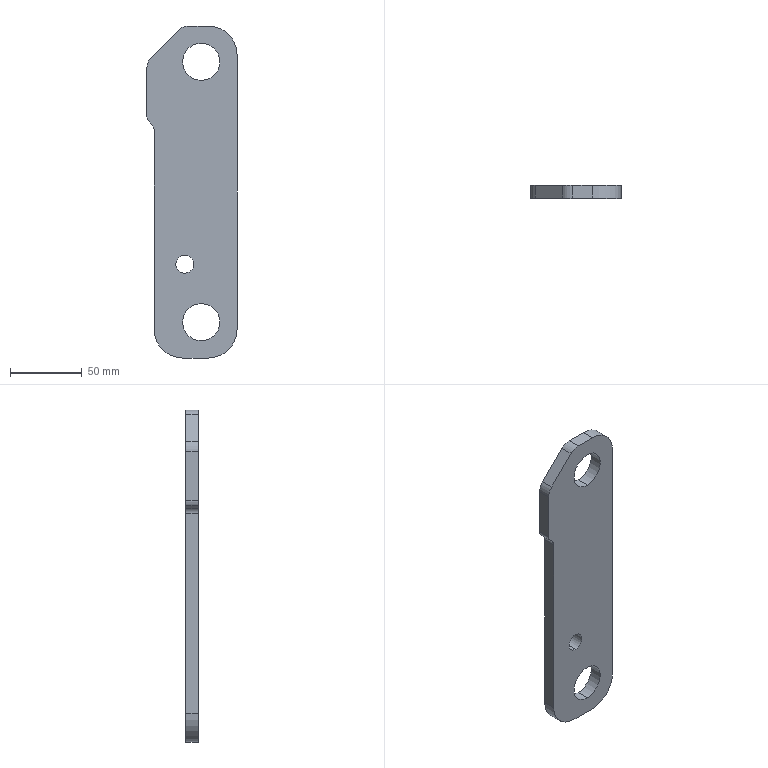Part | SolidWorks | features Extrusion 1 | 1 solid | 22 faces | box 63 x 9 x 232 mm | volume 108334 mm3 | cylinder 13 | plane 9 | commonest cylinder face diameters 26 x4 40 x3 10 x2 12.5 x2 20 x2
STEP:
#1=CARTESIAN_POINT('',(26.5,9.,-172.75));
#2=VERTEX_POINT('',#1);
#3=CARTESIAN_POINT('',(26.5,9.,-160.25));
#4=VERTEX_POINT('',#3);
#5=CARTESIAN_POINT('',(26.5,9.,-166.5));
#6=DIRECTION('',(0.,1.,0.));
#7=DIRECTION('',(0.,0.,1.));
#8=AXIS2_PLACEMENT_3D('',#5,#6,#7);
#9=CIRCLE('',#8,6.25);
#10=EDGE_CURVE('',#2,#4,#9,.T.);
#11=ORIENTED_EDGE('',*,*,#10,.T.);
#12=CARTESIAN_POINT('',(26.5,0.,-160.25));
#13=VERTEX_POINT('',#12);
#14=CARTESIAN_POINT('',(26.5,9.,-160.25));
#15=DIRECTION('',(0.,-1.,0.));
#16=VECTOR('',#15,1000.);
#17=LINE('',#14,#16);
#18=EDGE_CURVE('',#4,#13,#17,.T.);
#19=ORIENTED_EDGE('',*,*,#18,.T.);
#20=CARTESIAN_POINT('',(26.5,0.,-172.75));
#21=VERTEX_POINT('',#20);
#22=CARTESIAN_POINT('',(26.5,0.,-166.5));
#23=DIRECTION('',(0.,1.,0.));
#24=DIRECTION('',(0.,0.,1.));
#25=AXIS2_PLACEMENT_3D('',#22,#23,#24);
#26=CIRCLE('',#25,6.25);
#27=EDGE_CURVE('',#21,#13,#26,.T.);
#28=ORIENTED_EDGE('',*,*,#27,.F.);
#29=CARTESIAN_POINT('',(26.5,9.,-172.75));
#30=DIRECTION('',(0.,-1.,0.));
#31=VECTOR('',#30,1000.);
#32=LINE('',#29,#31);
#33=EDGE_CURVE('',#2,#21,#32,.T.);
#34=ORIENTED_EDGE('',*,*,#33,.F.);
#35=EDGE_LOOP('',(#11,#19,#28,#34));
#36=FACE_OUTER_BOUND('',#35,.T.);
#37=CARTESIAN_POINT('',(26.5,9.,-166.5));
#38=DIRECTION('',(0.,-1.,0.));
#39=DIRECTION('',(0.,0.,-1.));
#40=AXIS2_PLACEMENT_3D('',#37,#38,#39);
#41=CYLINDRICAL_SURFACE('',#40,6.25);
#42=ADVANCED_FACE('',(#36),#41,.F.);
#43=CARTESIAN_POINT('',(38.,9.,-220.));
#44=VERTEX_POINT('',#43);
#45=CARTESIAN_POINT('',(38.,9.,-194.));
#46=VERTEX_POINT('',#45);
#47=CARTESIAN_POINT('',(38.,9.,-207.));
#48=DIRECTION('',(0.,1.,0.));
#49=DIRECTION('',(0.,0.,1.));
#50=AXIS2_PLACEMENT_3D('',#47,#48,#49);
#51=CIRCLE('',#50,13.);
#52=EDGE_CURVE('',#44,#46,#51,.T.);
#53=ORIENTED_EDGE('',*,*,#52,.T.);
#54=CARTESIAN_POINT('',(38.,0.,-194.));
#55=VERTEX_POINT('',#54);
#56=CARTESIAN_POINT('',(38.,9.,-194.));
#57=DIRECTION('',(0.,-1.,0.));
#58=VECTOR('',#57,1000.);
#59=LINE('',#56,#58);
#60=EDGE_CURVE('',#46,#55,#59,.T.);
#61=ORIENTED_EDGE('',*,*,#60,.T.);
#62=CARTESIAN_POINT('',(38.,0.,-220.));
#63=VERTEX_POINT('',#62);
#64=CARTESIAN_POINT('',(38.,0.,-207.));
#65=DIRECTION('',(0.,1.,0.));
#66=DIRECTION('',(0.,0.,1.));
#67=AXIS2_PLACEMENT_3D('',#64,#65,#66);
#68=CIRCLE('',#67,13.);
#69=EDGE_CURVE('',#63,#55,#68,.T.);
#70=ORIENTED_EDGE('',*,*,#69,.F.);
#71=CARTESIAN_POINT('',(38.,9.,-220.));
#72=DIRECTION('',(0.,-1.,0.));
#73=VECTOR('',#72,1000.);
#74=LINE('',#71,#73);
#75=EDGE_CURVE('',#44,#63,#74,.T.);
#76=ORIENTED_EDGE('',*,*,#75,.F.);
#77=EDGE_LOOP('',(#53,#61,#70,#76));
#78=FACE_OUTER_BOUND('',#77,.T.);
#79=CARTESIAN_POINT('',(38.,9.,-207.));
#80=DIRECTION('',(0.,-1.,0.));
#81=DIRECTION('',(0.,0.,-1.));
#82=AXIS2_PLACEMENT_3D('',#79,#80,#81);
#83=CYLINDRICAL_SURFACE('',#82,13.);
#84=ADVANCED_FACE('',(#78),#83,.F.);
#85=CARTESIAN_POINT('',(38.,9.,-38.));
#86=VERTEX_POINT('',#85);
#87=CARTESIAN_POINT('',(38.,9.,-12.));
#88=VERTEX_POINT('',#87);
#89=CARTESIAN_POINT('',(38.,9.,-25.));
#90=DIRECTION('',(0.,1.,0.));
#91=DIRECTION('',(0.,0.,1.));
#92=AXIS2_PLACEMENT_3D('',#89,#90,#91);
#93=CIRCLE('',#92,13.);
#94=EDGE_CURVE('',#86,#88,#93,.T.);
#95=ORIENTED_EDGE('',*,*,#94,.T.);
#96=CARTESIAN_POINT('',(38.,0.,-12.));
#97=VERTEX_POINT('',#96);
#98=CARTESIAN_POINT('',(38.,9.,-12.));
#99=DIRECTION('',(0.,-1.,0.));
#100=VECTOR('',#99,1000.);
#101=LINE('',#98,#100);
#102=EDGE_CURVE('',#88,#97,#101,.T.);
#103=ORIENTED_EDGE('',*,*,#102,.T.);
#104=CARTESIAN_POINT('',(38.,0.,-38.));
#105=VERTEX_POINT('',#104);
#106=CARTESIAN_POINT('',(38.,0.,-25.));
#107=DIRECTION('',(0.,1.,0.));
#108=DIRECTION('',(0.,0.,1.));
#109=AXIS2_PLACEMENT_3D('',#106,#107,#108);
#110=CIRCLE('',#109,13.);
#111=EDGE_CURVE('',#105,#97,#110,.T.);
#112=ORIENTED_EDGE('',*,*,#111,.F.);
#113=CARTESIAN_POINT('',(38.,9.,-38.));
#114=DIRECTION('',(0.,-1.,0.));
#115=VECTOR('',#114,1000.);
#116=LINE('',#113,#115);
#117=EDGE_CURVE('',#86,#105,#116,.T.);
#118=ORIENTED_EDGE('',*,*,#117,.F.);
#119=EDGE_LOOP('',(#95,#103,#112,#118));
#120=FACE_OUTER_BOUND('',#119,.T.);
#121=CARTESIAN_POINT('',(38.,9.,-25.));
#122=DIRECTION('',(0.,-1.,0.));
#123=DIRECTION('',(0.,0.,-1.));
#124=AXIS2_PLACEMENT_3D('',#121,#122,#123);
#125=CYLINDRICAL_SURFACE('',#124,13.);
#126=ADVANCED_FACE('',(#120),#125,.F.);
#127=ORIENTED_EDGE('',*,*,#52,.F.);
#128=CARTESIAN_POINT('',(38.,9.,-207.));
#129=DIRECTION('',(0.,1.,0.));
#130=DIRECTION('',(0.,0.,1.));
#131=AXIS2_PLACEMENT_3D('',#128,#129,#130);
#132=CIRCLE('',#131,13.);
#133=EDGE_CURVE('',#46,#44,#132,.T.);
#134=ORIENTED_EDGE('',*,*,#133,.F.);
#135=EDGE_LOOP('',(#127,#134));
#136=FACE_BOUND('',#135,.T.);
#137=CARTESIAN_POINT('',(5.,9.,-72.571));
#138=VERTEX_POINT('',#137);
#139=CARTESIAN_POINT('',(3.536,9.,-69.036));
#140=VERTEX_POINT('',#139);
#141=CARTESIAN_POINT('',(0.,9.,-72.571));
#142=DIRECTION('',(0.,-1.,0.));
#143=DIRECTION('',(0.,0.,1.));
#144=AXIS2_PLACEMENT_3D('',#141,#142,#143);
#145=CIRCLE('',#144,5.);
#146=EDGE_CURVE('',#138,#140,#145,.T.);
#147=ORIENTED_EDGE('',*,*,#146,.T.);
#148=CARTESIAN_POINT('',(1.464,9.,-66.964));
#149=VERTEX_POINT('',#148);
#150=CARTESIAN_POINT('',(1.464,9.,-66.964));
#151=DIRECTION('',(-0.7071,0.,0.7071));
#152=VECTOR('',#151,1000.);
#153=LINE('',#150,#152);
#154=EDGE_CURVE('',#140,#149,#153,.T.);
#155=ORIENTED_EDGE('',*,*,#154,.T.);
#156=CARTESIAN_POINT('',(0.,9.,-63.429));
#157=VERTEX_POINT('',#156);
#158=CARTESIAN_POINT('',(5.,9.,-63.429));
#159=DIRECTION('',(0.,1.,0.));
#160=DIRECTION('',(0.,0.,-1.));
#161=AXIS2_PLACEMENT_3D('',#158,#159,#160);
#162=CIRCLE('',#161,5.);
#163=EDGE_CURVE('',#149,#157,#162,.T.);
#164=ORIENTED_EDGE('',*,*,#163,.T.);
#165=CARTESIAN_POINT('',(0.,9.,-29.142));
#166=VERTEX_POINT('',#165);
#167=CARTESIAN_POINT('',(0.,9.,-29.142));
#168=DIRECTION('',(0.,0.,1.));
#169=VECTOR('',#168,1000.);
#170=LINE('',#167,#169);
#171=EDGE_CURVE('',#157,#166,#170,.T.);
#172=ORIENTED_EDGE('',*,*,#171,.T.);
#173=CARTESIAN_POINT('',(2.929,9.,-22.071));
#174=VERTEX_POINT('',#173);
#175=CARTESIAN_POINT('',(10.,9.,-29.142));
#176=DIRECTION('',(0.,1.,0.));
#177=DIRECTION('',(0.,0.,-1.));
#178=AXIS2_PLACEMENT_3D('',#175,#176,#177);
#179=CIRCLE('',#178,10.);
#180=EDGE_CURVE('',#166,#174,#179,.T.);
#181=ORIENTED_EDGE('',*,*,#180,.T.);
#182=CARTESIAN_POINT('',(22.071,9.,-2.929));
#183=VERTEX_POINT('',#182);
#184=CARTESIAN_POINT('',(2.929,9.,-22.071));
#185=DIRECTION('',(0.7071,0.,0.7071));
#186=VECTOR('',#185,1000.);
#187=LINE('',#184,#186);
#188=EDGE_CURVE('',#174,#183,#187,.T.);
#189=ORIENTED_EDGE('',*,*,#188,.T.);
#190=CARTESIAN_POINT('',(29.142,9.,0.));
#191=VERTEX_POINT('',#190);
#192=CARTESIAN_POINT('',(29.142,9.,-10.));
#193=DIRECTION('',(0.,1.,0.));
#194=DIRECTION('',(0.,0.,1.));
#195=AXIS2_PLACEMENT_3D('',#192,#193,#194);
#196=CIRCLE('',#195,10.);
#197=EDGE_CURVE('',#183,#191,#196,.T.);
#198=ORIENTED_EDGE('',*,*,#197,.T.);
#199=CARTESIAN_POINT('',(43.,9.,0.));
#200=VERTEX_POINT('',#199);
#201=CARTESIAN_POINT('',(29.142,9.,0.));
#202=DIRECTION('',(1.,0.,0.));
#203=VECTOR('',#202,1000.);
#204=LINE('',#201,#203);
#205=EDGE_CURVE('',#191,#200,#204,.T.);
#206=ORIENTED_EDGE('',*,*,#205,.T.);
#207=CARTESIAN_POINT('',(63.,9.,-20.));
#208=VERTEX_POINT('',#207);
#209=CARTESIAN_POINT('',(43.,9.,-20.));
#210=DIRECTION('',(0.,1.,0.));
#211=DIRECTION('',(0.,0.,-1.));
#212=AXIS2_PLACEMENT_3D('',#209,#210,#211);
#213=CIRCLE('',#212,20.);
#214=EDGE_CURVE('',#200,#208,#213,.T.);
#215=ORIENTED_EDGE('',*,*,#214,.T.);
#216=CARTESIAN_POINT('',(63.,9.,-212.));
#217=VERTEX_POINT('',#216);
#218=CARTESIAN_POINT('',(63.,9.,-20.));
#219=DIRECTION('',(0.,0.,-1.));
#220=VECTOR('',#219,1000.);
#221=LINE('',#218,#220);
#222=EDGE_CURVE('',#208,#217,#221,.T.);
#223=ORIENTED_EDGE('',*,*,#222,.T.);
#224=CARTESIAN_POINT('',(43.,9.,-232.));
#225=VERTEX_POINT('',#224);
#226=CARTESIAN_POINT('',(43.,9.,-212.));
#227=DIRECTION('',(0.,1.,0.));
#228=DIRECTION('',(0.,0.,1.));
#229=AXIS2_PLACEMENT_3D('',#226,#227,#228);
#230=CIRCLE('',#229,20.);
#231=EDGE_CURVE('',#217,#225,#230,.T.);
#232=ORIENTED_EDGE('',*,*,#231,.T.);
#233=CARTESIAN_POINT('',(25.,9.,-232.));
#234=VERTEX_POINT('',#233);
#235=CARTESIAN_POINT('',(25.,9.,-232.));
#236=DIRECTION('',(-1.,0.,0.));
#237=VECTOR('',#236,1000.);
#238=LINE('',#235,#237);
#239=EDGE_CURVE('',#225,#234,#238,.T.);
#240=ORIENTED_EDGE('',*,*,#239,.T.);
#241=CARTESIAN_POINT('',(5.,9.,-212.));
#242=VERTEX_POINT('',#241);
#243=CARTESIAN_POINT('',(25.,9.,-212.));
#244=DIRECTION('',(0.,1.,0.));
#245=DIRECTION('',(0.,0.,-1.));
#246=AXIS2_PLACEMENT_3D('',#243,#244,#245);
#247=CIRCLE('',#246,20.);
#248=EDGE_CURVE('',#234,#242,#247,.T.);
#249=ORIENTED_EDGE('',*,*,#248,.T.);
#250=CARTESIAN_POINT('',(5.,9.,-72.571));
#251=DIRECTION('',(0.,0.,1.));
#252=VECTOR('',#251,1000.);
#253=LINE('',#250,#252);
#254=EDGE_CURVE('',#242,#138,#253,.T.);
#255=ORIENTED_EDGE('',*,*,#254,.T.);
#256=EDGE_LOOP('',(#147,#155,#164,#172,#181,#189,#198,#206,#215,#223,#232,#240,#249,#255));
#257=FACE_OUTER_BOUND('',#256,.T.);
#258=ORIENTED_EDGE('',*,*,#94,.F.);
#259=CARTESIAN_POINT('',(38.,9.,-25.));
#260=DIRECTION('',(0.,1.,0.));
#261=DIRECTION('',(0.,0.,1.));
#262=AXIS2_PLACEMENT_3D('',#259,#260,#261);
#263=CIRCLE('',#262,13.);
#264=EDGE_CURVE('',#88,#86,#263,.T.);
#265=ORIENTED_EDGE('',*,*,#264,.F.);
#266=EDGE_LOOP('',(#258,#265));
#267=FACE_BOUND('',#266,.T.);
#268=ORIENTED_EDGE('',*,*,#10,.F.);
#269=CARTESIAN_POINT('',(26.5,9.,-166.5));
#270=DIRECTION('',(0.,1.,0.));
#271=DIRECTION('',(0.,0.,1.));
#272=AXIS2_PLACEMENT_3D('',#269,#270,#271);
#273=CIRCLE('',#272,6.25);
#274=EDGE_CURVE('',#4,#2,#273,.T.);
#275=ORIENTED_EDGE('',*,*,#274,.F.);
#276=EDGE_LOOP('',(#268,#275));
#277=FACE_BOUND('',#276,.T.);
#278=CARTESIAN_POINT('',(0.,9.,-72.571));
#279=DIRECTION('',(0.,1.,0.));
#280=DIRECTION('',(0.,0.,1.));
#281=AXIS2_PLACEMENT_3D('',#278,#279,#280);
#282=PLANE('',#281);
#283=ADVANCED_FACE('',(#136,#257,#267,#277),#282,.T.);
#284=CARTESIAN_POINT('',(5.,0.,-72.571));
#285=VERTEX_POINT('',#284);
#286=CARTESIAN_POINT('',(3.536,0.,-69.036));
#287=VERTEX_POINT('',#286);
#288=CARTESIAN_POINT('',(0.,0.,-72.571));
#289=DIRECTION('',(0.,-1.,0.));
#290=DIRECTION('',(0.,0.,1.));
#291=AXIS2_PLACEMENT_3D('',#288,#289,#290);
#292=CIRCLE('',#291,5.);
#293=EDGE_CURVE('',#285,#287,#292,.T.);
#294=ORIENTED_EDGE('',*,*,#293,.F.);
#295=CARTESIAN_POINT('',(5.,0.,-212.));
#296=VERTEX_POINT('',#295);
#297=CARTESIAN_POINT('',(5.,0.,-72.571));
#298=DIRECTION('',(0.,0.,1.));
#299=VECTOR('',#298,1000.);
#300=LINE('',#297,#299);
#301=EDGE_CURVE('',#296,#285,#300,.T.);
#302=ORIENTED_EDGE('',*,*,#301,.F.);
#303=CARTESIAN_POINT('',(25.,0.,-232.));
#304=VERTEX_POINT('',#303);
#305=CARTESIAN_POINT('',(25.,0.,-212.));
#306=DIRECTION('',(0.,1.,0.));
#307=DIRECTION('',(0.,0.,-1.));
#308=AXIS2_PLACEMENT_3D('',#305,#306,#307);
#309=CIRCLE('',#308,20.);
#310=EDGE_CURVE('',#304,#296,#309,.T.);
#311=ORIENTED_EDGE('',*,*,#310,.F.);
#312=CARTESIAN_POINT('',(43.,0.,-232.));
#313=VERTEX_POINT('',#312);
#314=CARTESIAN_POINT('',(25.,0.,-232.));
#315=DIRECTION('',(-1.,0.,0.));
#316=VECTOR('',#315,1000.);
#317=LINE('',#314,#316);
#318=EDGE_CURVE('',#313,#304,#317,.T.);
#319=ORIENTED_EDGE('',*,*,#318,.F.);
#320=CARTESIAN_POINT('',(63.,0.,-212.));
#321=VERTEX_POINT('',#320);
#322=CARTESIAN_POINT('',(43.,0.,-212.));
#323=DIRECTION('',(0.,1.,0.));
#324=DIRECTION('',(0.,0.,1.));
#325=AXIS2_PLACEMENT_3D('',#322,#323,#324);
#326=CIRCLE('',#325,20.);
#327=EDGE_CURVE('',#321,#313,#326,.T.);
#328=ORIENTED_EDGE('',*,*,#327,.F.);
#329=CARTESIAN_POINT('',(63.,0.,-20.));
#330=VERTEX_POINT('',#329);
#331=CARTESIAN_POINT('',(63.,0.,-20.));
#332=DIRECTION('',(0.,0.,-1.));
#333=VECTOR('',#332,1000.);
#334=LINE('',#331,#333);
#335=EDGE_CURVE('',#330,#321,#334,.T.);
#336=ORIENTED_EDGE('',*,*,#335,.F.);
#337=CARTESIAN_POINT('',(43.,0.,0.));
#338=VERTEX_POINT('',#337);
#339=CARTESIAN_POINT('',(43.,0.,-20.));
#340=DIRECTION('',(0.,1.,0.));
#341=DIRECTION('',(0.,0.,-1.));
#342=AXIS2_PLACEMENT_3D('',#339,#340,#341);
#343=CIRCLE('',#342,20.);
#344=EDGE_CURVE('',#338,#330,#343,.T.);
#345=ORIENTED_EDGE('',*,*,#344,.F.);
#346=CARTESIAN_POINT('',(29.142,0.,0.));
#347=VERTEX_POINT('',#346);
#348=CARTESIAN_POINT('',(29.142,0.,0.));
#349=DIRECTION('',(1.,0.,0.));
#350=VECTOR('',#349,1000.);
#351=LINE('',#348,#350);
#352=EDGE_CURVE('',#347,#338,#351,.T.);
#353=ORIENTED_EDGE('',*,*,#352,.F.);
#354=CARTESIAN_POINT('',(22.071,0.,-2.929));
#355=VERTEX_POINT('',#354);
#356=CARTESIAN_POINT('',(29.142,0.,-10.));
#357=DIRECTION('',(0.,1.,0.));
#358=DIRECTION('',(0.,0.,1.));
#359=AXIS2_PLACEMENT_3D('',#356,#357,#358);
#360=CIRCLE('',#359,10.);
#361=EDGE_CURVE('',#355,#347,#360,.T.);
#362=ORIENTED_EDGE('',*,*,#361,.F.);
#363=CARTESIAN_POINT('',(2.929,0.,-22.071));
#364=VERTEX_POINT('',#363);
#365=CARTESIAN_POINT('',(2.929,0.,-22.071));
#366=DIRECTION('',(0.7071,0.,0.7071));
#367=VECTOR('',#366,1000.);
#368=LINE('',#365,#367);
#369=EDGE_CURVE('',#364,#355,#368,.T.);
#370=ORIENTED_EDGE('',*,*,#369,.F.);
#371=CARTESIAN_POINT('',(0.,0.,-29.142));
#372=VERTEX_POINT('',#371);
#373=CARTESIAN_POINT('',(10.,0.,-29.142));
#374=DIRECTION('',(0.,1.,0.));
#375=DIRECTION('',(0.,0.,-1.));
#376=AXIS2_PLACEMENT_3D('',#373,#374,#375);
#377=CIRCLE('',#376,10.);
#378=EDGE_CURVE('',#372,#364,#377,.T.);
#379=ORIENTED_EDGE('',*,*,#378,.F.);
#380=CARTESIAN_POINT('',(0.,0.,-63.429));
#381=VERTEX_POINT('',#380);
#382=CARTESIAN_POINT('',(0.,0.,-29.142));
#383=DIRECTION('',(0.,0.,1.));
#384=VECTOR('',#383,1000.);
#385=LINE('',#382,#384);
#386=EDGE_CURVE('',#381,#372,#385,.T.);
#387=ORIENTED_EDGE('',*,*,#386,.F.);
#388=CARTESIAN_POINT('',(1.464,0.,-66.964));
#389=VERTEX_POINT('',#388);
#390=CARTESIAN_POINT('',(5.,0.,-63.429));
#391=DIRECTION('',(0.,1.,0.));
#392=DIRECTION('',(0.,0.,-1.));
#393=AXIS2_PLACEMENT_3D('',#390,#391,#392);
#394=CIRCLE('',#393,5.);
#395=EDGE_CURVE('',#389,#381,#394,.T.);
#396=ORIENTED_EDGE('',*,*,#395,.F.);
#397=CARTESIAN_POINT('',(1.464,0.,-66.964));
#398=DIRECTION('',(-0.7071,0.,0.7071));
#399=VECTOR('',#398,1000.);
#400=LINE('',#397,#399);
#401=EDGE_CURVE('',#287,#389,#400,.T.);
#402=ORIENTED_EDGE('',*,*,#401,.F.);
#403=EDGE_LOOP('',(#294,#302,#311,#319,#328,#336,#345,#353,#362,#370,#379,#387,#396,#402));
#404=FACE_OUTER_BOUND('',#403,.T.);
#405=ORIENTED_EDGE('',*,*,#111,.T.);
#406=CARTESIAN_POINT('',(38.,0.,-25.));
#407=DIRECTION('',(0.,1.,0.));
#408=DIRECTION('',(0.,0.,1.));
#409=AXIS2_PLACEMENT_3D('',#406,#407,#408);
#410=CIRCLE('',#409,13.);
#411=EDGE_CURVE('',#97,#105,#410,.T.);
#412=ORIENTED_EDGE('',*,*,#411,.T.);
#413=EDGE_LOOP('',(#405,#412));
#414=FACE_BOUND('',#413,.T.);
#415=ORIENTED_EDGE('',*,*,#69,.T.);
#416=CARTESIAN_POINT('',(38.,0.,-207.));
#417=DIRECTION('',(0.,1.,0.));
#418=DIRECTION('',(0.,0.,1.));
#419=AXIS2_PLACEMENT_3D('',#416,#417,#418);
#420=CIRCLE('',#419,13.);
#421=EDGE_CURVE('',#55,#63,#420,.T.);
#422=ORIENTED_EDGE('',*,*,#421,.T.);
#423=EDGE_LOOP('',(#415,#422));
#424=FACE_BOUND('',#423,.T.);
#425=ORIENTED_EDGE('',*,*,#27,.T.);
#426=CARTESIAN_POINT('',(26.5,0.,-166.5));
#427=DIRECTION('',(0.,1.,0.));
#428=DIRECTION('',(0.,0.,1.));
#429=AXIS2_PLACEMENT_3D('',#426,#427,#428);
#430=CIRCLE('',#429,6.25);
#431=EDGE_CURVE('',#13,#21,#430,.T.);
#432=ORIENTED_EDGE('',*,*,#431,.T.);
#433=EDGE_LOOP('',(#425,#432));
#434=FACE_BOUND('',#433,.T.);
#435=CARTESIAN_POINT('',(0.,0.,-72.571));
#436=DIRECTION('',(0.,1.,0.));
#437=DIRECTION('',(0.,0.,1.));
#438=AXIS2_PLACEMENT_3D('',#435,#436,#437);
#439=PLANE('',#438);
#440=ADVANCED_FACE('',(#404,#414,#424,#434),#439,.F.);
#441=ORIENTED_EDGE('',*,*,#293,.T.);
#442=CARTESIAN_POINT('',(3.536,9.,-69.036));
#443=DIRECTION('',(0.,-1.,0.));
#444=VECTOR('',#443,1000.);
#445=LINE('',#442,#444);
#446=EDGE_CURVE('',#140,#287,#445,.T.);
#447=ORIENTED_EDGE('',*,*,#446,.F.);
#448=ORIENTED_EDGE('',*,*,#146,.F.);
#449=CARTESIAN_POINT('',(5.,9.,-72.571));
#450=DIRECTION('',(0.,-1.,0.));
#451=VECTOR('',#450,1000.);
#452=LINE('',#449,#451);
#453=EDGE_CURVE('',#138,#285,#452,.T.);
#454=ORIENTED_EDGE('',*,*,#453,.T.);
#455=EDGE_LOOP('',(#441,#447,#448,#454));
#456=FACE_OUTER_BOUND('',#455,.T.);
#457=CARTESIAN_POINT('',(0.,9.,-72.571));
#458=DIRECTION('',(0.,-1.,0.));
#459=DIRECTION('',(0.,0.,-1.));
#460=AXIS2_PLACEMENT_3D('',#457,#458,#459);
#461=CYLINDRICAL_SURFACE('',#460,5.);
#462=ADVANCED_FACE('',(#456),#461,.F.);
#463=ORIENTED_EDGE('',*,*,#401,.T.);
#464=CARTESIAN_POINT('',(1.464,9.,-66.964));
#465=DIRECTION('',(0.,-1.,0.));
#466=VECTOR('',#465,1000.);
#467=LINE('',#464,#466);
#468=EDGE_CURVE('',#149,#389,#467,.T.);
#469=ORIENTED_EDGE('',*,*,#468,.F.);
#470=ORIENTED_EDGE('',*,*,#154,.F.);
#471=ORIENTED_EDGE('',*,*,#446,.T.);
#472=EDGE_LOOP('',(#463,#469,#470,#471));
#473=FACE_OUTER_BOUND('',#472,.T.);
#474=CARTESIAN_POINT('',(1.464,9.,-66.964));
#475=DIRECTION('',(0.7071,0.,0.7071));
#476=DIRECTION('',(0.7071,0.,-0.7071));
#477=AXIS2_PLACEMENT_3D('',#474,#475,#476);
#478=PLANE('',#477);
#479=ADVANCED_FACE('',(#473),#478,.F.);
#480=ORIENTED_EDGE('',*,*,#395,.T.);
#481=CARTESIAN_POINT('',(0.,9.,-63.429));
#482=DIRECTION('',(0.,-1.,0.));
#483=VECTOR('',#482,1000.);
#484=LINE('',#481,#483);
#485=EDGE_CURVE('',#157,#381,#484,.T.);
#486=ORIENTED_EDGE('',*,*,#485,.F.);
#487=ORIENTED_EDGE('',*,*,#163,.F.);
#488=ORIENTED_EDGE('',*,*,#468,.T.);
#489=EDGE_LOOP('',(#480,#486,#487,#488));
#490=FACE_OUTER_BOUND('',#489,.T.);
#491=CARTESIAN_POINT('',(5.,9.,-63.429));
#492=DIRECTION('',(0.,-1.,0.));
#493=DIRECTION('',(0.,0.,-1.));
#494=AXIS2_PLACEMENT_3D('',#491,#492,#493);
#495=CYLINDRICAL_SURFACE('',#494,5.);
#496=ADVANCED_FACE('',(#490),#495,.T.);
#497=ORIENTED_EDGE('',*,*,#386,.T.);
#498=CARTESIAN_POINT('',(0.,9.,-29.142));
#499=DIRECTION('',(0.,-1.,0.));
#500=VECTOR('',#499,1000.);
#501=LINE('',#498,#500);
#502=EDGE_CURVE('',#166,#372,#501,.T.);
#503=ORIENTED_EDGE('',*,*,#502,.F.);
#504=ORIENTED_EDGE('',*,*,#171,.F.);
#505=ORIENTED_EDGE('',*,*,#485,.T.);
#506=EDGE_LOOP('',(#497,#503,#504,#505));
#507=FACE_OUTER_BOUND('',#506,.T.);
#508=CARTESIAN_POINT('',(0.,9.,-29.142));
#509=DIRECTION('',(1.,0.,0.));
#510=DIRECTION('',(0.,0.,-1.));
#511=AXIS2_PLACEMENT_3D('',#508,#509,#510);
#512=PLANE('',#511);
#513=ADVANCED_FACE('',(#507),#512,.F.);
#514=ORIENTED_EDGE('',*,*,#378,.T.);
#515=CARTESIAN_POINT('',(2.929,9.,-22.071));
#516=DIRECTION('',(0.,-1.,0.));
#517=VECTOR('',#516,1000.);
#518=LINE('',#515,#517);
#519=EDGE_CURVE('',#174,#364,#518,.T.);
#520=ORIENTED_EDGE('',*,*,#519,.F.);
#521=ORIENTED_EDGE('',*,*,#180,.F.);
#522=ORIENTED_EDGE('',*,*,#502,.T.);
#523=EDGE_LOOP('',(#514,#520,#521,#522));
#524=FACE_OUTER_BOUND('',#523,.T.);
#525=CARTESIAN_POINT('',(10.,9.,-29.142));
#526=DIRECTION('',(0.,-1.,0.));
#527=DIRECTION('',(0.,0.,-1.));
#528=AXIS2_PLACEMENT_3D('',#525,#526,#527);
#529=CYLINDRICAL_SURFACE('',#528,10.);
#530=ADVANCED_FACE('',(#524),#529,.T.);
#531=ORIENTED_EDGE('',*,*,#369,.T.);
#532=CARTESIAN_POINT('',(22.071,9.,-2.929));
#533=DIRECTION('',(0.,-1.,0.));
#534=VECTOR('',#533,1000.);
#535=LINE('',#532,#534);
#536=EDGE_CURVE('',#183,#355,#535,.T.);
#537=ORIENTED_EDGE('',*,*,#536,.F.);
#538=ORIENTED_EDGE('',*,*,#188,.F.);
#539=ORIENTED_EDGE('',*,*,#519,.T.);
#540=EDGE_LOOP('',(#531,#537,#538,#539));
#541=FACE_OUTER_BOUND('',#540,.T.);
#542=CARTESIAN_POINT('',(2.929,9.,-22.071));
#543=DIRECTION('',(0.7071,0.,-0.7071));
#544=DIRECTION('',(-0.7071,0.,-0.7071));
#545=AXIS2_PLACEMENT_3D('',#542,#543,#544);
#546=PLANE('',#545);
#547=ADVANCED_FACE('',(#541),#546,.F.);
#548=ORIENTED_EDGE('',*,*,#361,.T.);
#549=CARTESIAN_POINT('',(29.142,9.,0.));
#550=DIRECTION('',(0.,-1.,0.));
#551=VECTOR('',#550,1000.);
#552=LINE('',#549,#551);
#553=EDGE_CURVE('',#191,#347,#552,.T.);
#554=ORIENTED_EDGE('',*,*,#553,.F.);
#555=ORIENTED_EDGE('',*,*,#197,.F.);
#556=ORIENTED_EDGE('',*,*,#536,.T.);
#557=EDGE_LOOP('',(#548,#554,#555,#556));
#558=FACE_OUTER_BOUND('',#557,.T.);
#559=CARTESIAN_POINT('',(29.142,9.,-10.));
#560=DIRECTION('',(0.,-1.,0.));
#561=DIRECTION('',(0.,0.,-1.));
#562=AXIS2_PLACEMENT_3D('',#559,#560,#561);
#563=CYLINDRICAL_SURFACE('',#562,10.);
#564=ADVANCED_FACE('',(#558),#563,.T.);
#565=ORIENTED_EDGE('',*,*,#352,.T.);
#566=CARTESIAN_POINT('',(43.,9.,0.));
#567=DIRECTION('',(0.,-1.,0.));
#568=VECTOR('',#567,1000.);
#569=LINE('',#566,#568);
#570=EDGE_CURVE('',#200,#338,#569,.T.);
#571=ORIENTED_EDGE('',*,*,#570,.F.);
#572=ORIENTED_EDGE('',*,*,#205,.F.);
#573=ORIENTED_EDGE('',*,*,#553,.T.);
#574=EDGE_LOOP('',(#565,#571,#572,#573));
#575=FACE_OUTER_BOUND('',#574,.T.);
#576=CARTESIAN_POINT('',(29.142,9.,0.));
#577=DIRECTION('',(0.,0.,-1.));
#578=DIRECTION('',(-1.,0.,0.));
#579=AXIS2_PLACEMENT_3D('',#576,#577,#578);
#580=PLANE('',#579);
#581=ADVANCED_FACE('',(#575),#580,.F.);
#582=ORIENTED_EDGE('',*,*,#344,.T.);
#583=CARTESIAN_POINT('',(63.,9.,-20.));
#584=DIRECTION('',(0.,-1.,0.));
#585=VECTOR('',#584,1000.);
#586=LINE('',#583,#585);
#587=EDGE_CURVE('',#208,#330,#586,.T.);
#588=ORIENTED_EDGE('',*,*,#587,.F.);
#589=ORIENTED_EDGE('',*,*,#214,.F.);
#590=ORIENTED_EDGE('',*,*,#570,.T.);
#591=EDGE_LOOP('',(#582,#588,#589,#590));
#592=FACE_OUTER_BOUND('',#591,.T.);
#593=CARTESIAN_POINT('',(43.,9.,-20.));
#594=DIRECTION('',(0.,-1.,0.));
#595=DIRECTION('',(0.,0.,-1.));
#596=AXIS2_PLACEMENT_3D('',#593,#594,#595);
#597=CYLINDRICAL_SURFACE('',#596,20.);
#598=ADVANCED_FACE('',(#592),#597,.T.);
#599=ORIENTED_EDGE('',*,*,#335,.T.);
#600=CARTESIAN_POINT('',(63.,9.,-212.));
#601=DIRECTION('',(0.,-1.,0.));
#602=VECTOR('',#601,1000.);
#603=LINE('',#600,#602);
#604=EDGE_CURVE('',#217,#321,#603,.T.);
#605=ORIENTED_EDGE('',*,*,#604,.F.);
#606=ORIENTED_EDGE('',*,*,#222,.F.);
#607=ORIENTED_EDGE('',*,*,#587,.T.);
#608=EDGE_LOOP('',(#599,#605,#606,#607));
#609=FACE_OUTER_BOUND('',#608,.T.);
#610=CARTESIAN_POINT('',(63.,9.,-20.));
#611=DIRECTION('',(-1.,0.,0.));
#612=DIRECTION('',(0.,0.,1.));
#613=AXIS2_PLACEMENT_3D('',#610,#611,#612);
#614=PLANE('',#613);
#615=ADVANCED_FACE('',(#609),#614,.F.);
#616=ORIENTED_EDGE('',*,*,#327,.T.);
#617=CARTESIAN_POINT('',(43.,9.,-232.));
#618=DIRECTION('',(0.,-1.,0.));
#619=VECTOR('',#618,1000.);
#620=LINE('',#617,#619);
#621=EDGE_CURVE('',#225,#313,#620,.T.);
#622=ORIENTED_EDGE('',*,*,#621,.F.);
#623=ORIENTED_EDGE('',*,*,#231,.F.);
#624=ORIENTED_EDGE('',*,*,#604,.T.);
#625=EDGE_LOOP('',(#616,#622,#623,#624));
#626=FACE_OUTER_BOUND('',#625,.T.);
#627=CARTESIAN_POINT('',(43.,9.,-212.));
#628=DIRECTION('',(0.,-1.,0.));
#629=DIRECTION('',(0.,0.,-1.));
#630=AXIS2_PLACEMENT_3D('',#627,#628,#629);
#631=CYLINDRICAL_SURFACE('',#630,20.);
#632=ADVANCED_FACE('',(#626),#631,.T.);
#633=ORIENTED_EDGE('',*,*,#318,.T.);
#634=CARTESIAN_POINT('',(25.,9.,-232.));
#635=DIRECTION('',(0.,-1.,0.));
#636=VECTOR('',#635,1000.);
#637=LINE('',#634,#636);
#638=EDGE_CURVE('',#234,#304,#637,.T.);
#639=ORIENTED_EDGE('',*,*,#638,.F.);
#640=ORIENTED_EDGE('',*,*,#239,.F.);
#641=ORIENTED_EDGE('',*,*,#621,.T.);
#642=EDGE_LOOP('',(#633,#639,#640,#641));
#643=FACE_OUTER_BOUND('',#642,.T.);
#644=CARTESIAN_POINT('',(25.,9.,-232.));
#645=DIRECTION('',(0.,0.,1.));
#646=DIRECTION('',(1.,0.,0.));
#647=AXIS2_PLACEMENT_3D('',#644,#645,#646);
#648=PLANE('',#647);
#649=ADVANCED_FACE('',(#643),#648,.F.);
#650=ORIENTED_EDGE('',*,*,#310,.T.);
#651=CARTESIAN_POINT('',(5.,9.,-212.));
#652=DIRECTION('',(0.,-1.,0.));
#653=VECTOR('',#652,1000.);
#654=LINE('',#651,#653);
#655=EDGE_CURVE('',#242,#296,#654,.T.);
#656=ORIENTED_EDGE('',*,*,#655,.F.);
#657=ORIENTED_EDGE('',*,*,#248,.F.);
#658=ORIENTED_EDGE('',*,*,#638,.T.);
#659=EDGE_LOOP('',(#650,#656,#657,#658));
#660=FACE_OUTER_BOUND('',#659,.T.);
#661=CARTESIAN_POINT('',(25.,9.,-212.));
#662=DIRECTION('',(0.,-1.,0.));
#663=DIRECTION('',(0.,0.,-1.));
#664=AXIS2_PLACEMENT_3D('',#661,#662,#663);
#665=CYLINDRICAL_SURFACE('',#664,20.);
#666=ADVANCED_FACE('',(#660),#665,.T.);
#667=ORIENTED_EDGE('',*,*,#301,.T.);
#668=ORIENTED_EDGE('',*,*,#453,.F.);
#669=ORIENTED_EDGE('',*,*,#254,.F.);
#670=ORIENTED_EDGE('',*,*,#655,.T.);
#671=EDGE_LOOP('',(#667,#668,#669,#670));
#672=FACE_OUTER_BOUND('',#671,.T.);
#673=CARTESIAN_POINT('',(5.,9.,-72.571));
#674=DIRECTION('',(1.,0.,0.));
#675=DIRECTION('',(0.,0.,-1.));
#676=AXIS2_PLACEMENT_3D('',#673,#674,#675);
#677=PLANE('',#676);
#678=ADVANCED_FACE('',(#672),#677,.F.);
#679=ORIENTED_EDGE('',*,*,#102,.F.);
#680=ORIENTED_EDGE('',*,*,#264,.T.);
#681=ORIENTED_EDGE('',*,*,#117,.T.);
#682=ORIENTED_EDGE('',*,*,#411,.F.);
#683=EDGE_LOOP('',(#679,#680,#681,#682));
#684=FACE_OUTER_BOUND('',#683,.T.);
#685=CARTESIAN_POINT('',(38.,9.,-25.));
#686=DIRECTION('',(0.,-1.,0.));
#687=DIRECTION('',(0.,0.,-1.));
#688=AXIS2_PLACEMENT_3D('',#685,#686,#687);
#689=CYLINDRICAL_SURFACE('',#688,13.);
#690=ADVANCED_FACE('',(#684),#689,.F.);
#691=ORIENTED_EDGE('',*,*,#60,.F.);
#692=ORIENTED_EDGE('',*,*,#133,.T.);
#693=ORIENTED_EDGE('',*,*,#75,.T.);
#694=ORIENTED_EDGE('',*,*,#421,.F.);
#695=EDGE_LOOP('',(#691,#692,#693,#694));
#696=FACE_OUTER_BOUND('',#695,.T.);
#697=CARTESIAN_POINT('',(38.,9.,-207.));
#698=DIRECTION('',(0.,-1.,0.));
#699=DIRECTION('',(0.,0.,-1.));
#700=AXIS2_PLACEMENT_3D('',#697,#698,#699);
#701=CYLINDRICAL_SURFACE('',#700,13.);
#702=ADVANCED_FACE('',(#696),#701,.F.);
#703=ORIENTED_EDGE('',*,*,#18,.F.);
#704=ORIENTED_EDGE('',*,*,#274,.T.);
#705=ORIENTED_EDGE('',*,*,#33,.T.);
#706=ORIENTED_EDGE('',*,*,#431,.F.);
#707=EDGE_LOOP('',(#703,#704,#705,#706));
#708=FACE_OUTER_BOUND('',#707,.T.);
#709=CARTESIAN_POINT('',(26.5,9.,-166.5));
#710=DIRECTION('',(0.,-1.,0.));
#711=DIRECTION('',(0.,0.,-1.));
#712=AXIS2_PLACEMENT_3D('',#709,#710,#711);
#713=CYLINDRICAL_SURFACE('',#712,6.25);
#714=ADVANCED_FACE('',(#708),#713,.F.);
#715=CLOSED_SHELL('',(#42,#84,#126,#283,#440,#462,#479,#496,#513,#530,#547,#564,#581,#598,#615,#632,#649,#666,#678,#690,#702,#714));
#716=MANIFOLD_SOLID_BREP('',#715);
#717=CARTESIAN_POINT('',(0.,0.,0.));
#718=DIRECTION('',(0.,0.,1.));
#719=DIRECTION('',(1.,0.,0.));
#720=AXIS2_PLACEMENT_3D('',#717,#718,#719);
#721=(LENGTH_UNIT()NAMED_UNIT(*)SI_UNIT(.MILLI.,.METRE.));
#722=UNCERTAINTY_MEASURE_WITH_UNIT(LENGTH_MEASURE(0.00001),#721,'','');
#723=(NAMED_UNIT(*)PLANE_ANGLE_UNIT()SI_UNIT($,.RADIAN.));
#724=(NAMED_UNIT(*)SI_UNIT($,.STERADIAN.)SOLID_ANGLE_UNIT());
#725=(GEOMETRIC_REPRESENTATION_CONTEXT(3)GLOBAL_UNCERTAINTY_ASSIGNED_CONTEXT((#722))GLOBAL_UNIT_ASSIGNED_CONTEXT((#721,#723,#724))REPRESENTATION_CONTEXT('',''));
#726=ADVANCED_BREP_SHAPE_REPRESENTATION('',(#716,#720),#725);